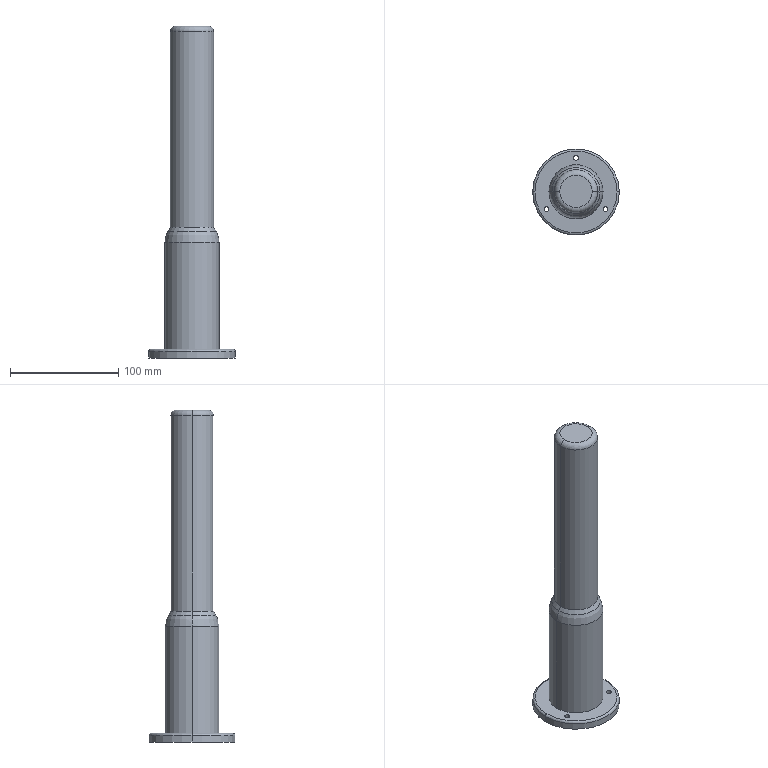Part | STEP file | QA-TPWB4-L73ROG | 1 solid | 23 faces | box 80 x 80 x 307 mm | volume 491038 mm3 | cylinder 12 | torus 4 | plane 3 | other 2 | cone 2 | commonest cylinder face diameters 4.5 x6 40 x2 50 x2 80 x2